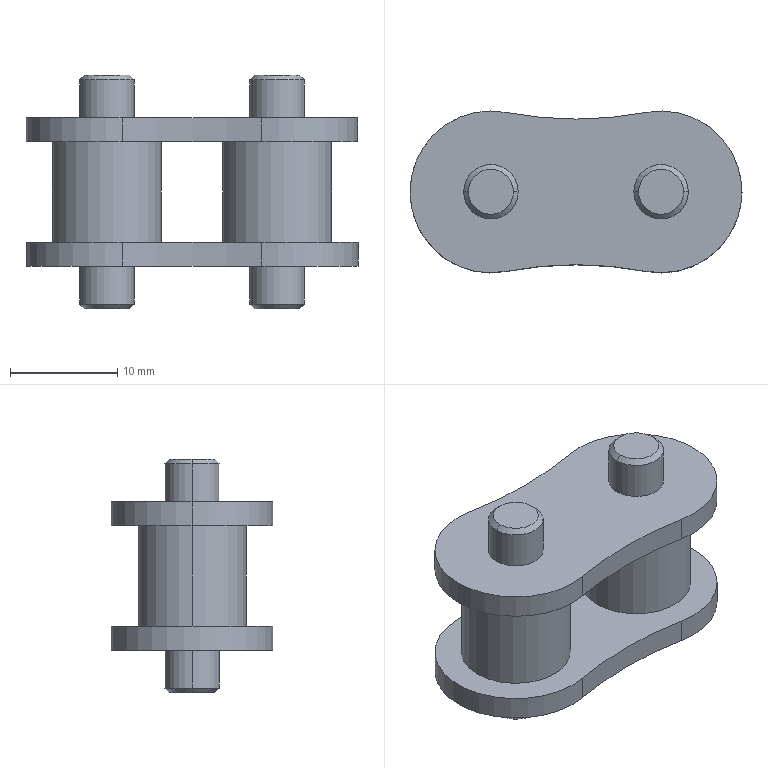Part | SolidWorks | features Boss 2, Chamfer 1, CompositeCurve 1, Extrusion 1, MirrorPattern 1 | 1 solid | 38 faces | box 30.965 x 15.09 x 21.8 mm | volume 3635 mm3 | cylinder 22 | cone 8 | plane 8 | commonest cylinder face diameters 5.09 x8 15.09 x6 10.16 x4 69.169 x4
STEP:
#1=CARTESIAN_POINT('',(-5.836,0.,10.9));
#2=VERTEX_POINT('',#1);
#3=CARTESIAN_POINT('',(-10.039,0.,10.9));
#4=VERTEX_POINT('',#3);
#5=CARTESIAN_POINT('',(-7.938,0.,10.9));
#6=DIRECTION('',(0.,0.,1.));
#7=DIRECTION('',(1.,0.,0.));
#8=AXIS2_PLACEMENT_3D('',#5,#6,#7);
#9=CIRCLE('',#8,2.101);
#10=EDGE_CURVE('',#2,#4,#9,.T.);
#11=ORIENTED_EDGE('',*,*,#10,.F.);
#12=CARTESIAN_POINT('',(-5.393,0.,10.456));
#13=VERTEX_POINT('',#12);
#14=CARTESIAN_POINT('',(-5.836,0.,10.9));
#15=DIRECTION('',(0.7071,0.,-0.7071));
#16=VECTOR('',#15,1000.);
#17=LINE('',#14,#16);
#18=EDGE_CURVE('',#2,#13,#17,.T.);
#19=ORIENTED_EDGE('',*,*,#18,.T.);
#20=CARTESIAN_POINT('',(-10.482,0.,10.456));
#21=VERTEX_POINT('',#20);
#22=CARTESIAN_POINT('',(-7.938,0.,10.456));
#23=DIRECTION('',(0.,0.,-1.));
#24=DIRECTION('',(1.,0.,0.));
#25=AXIS2_PLACEMENT_3D('',#22,#23,#24);
#26=CIRCLE('',#25,2.545);
#27=EDGE_CURVE('',#21,#13,#26,.T.);
#28=ORIENTED_EDGE('',*,*,#27,.F.);
#29=CARTESIAN_POINT('',(-10.039,0.,10.9));
#30=DIRECTION('',(-0.7071,0.,-0.7071));
#31=VECTOR('',#30,1000.);
#32=LINE('',#29,#31);
#33=EDGE_CURVE('',#4,#21,#32,.T.);
#34=ORIENTED_EDGE('',*,*,#33,.F.);
#35=EDGE_LOOP('',(#11,#19,#28,#34));
#36=FACE_OUTER_BOUND('',#35,.T.);
#37=CARTESIAN_POINT('',(-7.938,0.,10.9));
#38=DIRECTION('',(0.,0.,-1.));
#39=DIRECTION('',(-1.,0.,0.));
#40=AXIS2_PLACEMENT_3D('',#37,#38,#39);
#41=CONICAL_SURFACE('',#40,2.101,0.7854);
#42=ADVANCED_FACE('',(#36),#41,.T.);
#43=CARTESIAN_POINT('',(-10.038,0.,-10.9));
#44=VERTEX_POINT('',#43);
#45=CARTESIAN_POINT('',(-5.837,0.,-10.9));
#46=VERTEX_POINT('',#45);
#47=CARTESIAN_POINT('',(-7.938,0.,-10.9));
#48=DIRECTION('',(0.,0.,-1.));
#49=DIRECTION('',(1.,0.,0.));
#50=AXIS2_PLACEMENT_3D('',#47,#48,#49);
#51=CIRCLE('',#50,2.101);
#52=EDGE_CURVE('',#44,#46,#51,.T.);
#53=ORIENTED_EDGE('',*,*,#52,.F.);
#54=CARTESIAN_POINT('',(-10.482,0.,-10.456));
#55=VERTEX_POINT('',#54);
#56=CARTESIAN_POINT('',(-10.482,0.,-10.456));
#57=DIRECTION('',(-0.7071,0.,0.7071));
#58=VECTOR('',#57,1000.);
#59=LINE('',#56,#58);
#60=EDGE_CURVE('',#44,#55,#59,.T.);
#61=ORIENTED_EDGE('',*,*,#60,.T.);
#62=CARTESIAN_POINT('',(-5.393,0.,-10.456));
#63=VERTEX_POINT('',#62);
#64=CARTESIAN_POINT('',(-7.938,0.,-10.456));
#65=DIRECTION('',(0.,0.,1.));
#66=DIRECTION('',(1.,0.,0.));
#67=AXIS2_PLACEMENT_3D('',#64,#65,#66);
#68=CIRCLE('',#67,2.545);
#69=EDGE_CURVE('',#63,#55,#68,.T.);
#70=ORIENTED_EDGE('',*,*,#69,.F.);
#71=CARTESIAN_POINT('',(-5.393,0.,-10.456));
#72=DIRECTION('',(0.7071,0.,0.7071));
#73=VECTOR('',#72,1000.);
#74=LINE('',#71,#73);
#75=EDGE_CURVE('',#46,#63,#74,.T.);
#76=ORIENTED_EDGE('',*,*,#75,.F.);
#77=EDGE_LOOP('',(#53,#61,#70,#76));
#78=FACE_OUTER_BOUND('',#77,.T.);
#79=CARTESIAN_POINT('',(-7.938,0.,-10.456));
#80=DIRECTION('',(0.,0.,1.));
#81=DIRECTION('',(1.,0.,0.));
#82=AXIS2_PLACEMENT_3D('',#79,#80,#81);
#83=CONICAL_SURFACE('',#82,2.545,0.7854);
#84=ADVANCED_FACE('',(#78),#83,.T.);
#85=CARTESIAN_POINT('',(10.039,0.,10.9));
#86=VERTEX_POINT('',#85);
#87=CARTESIAN_POINT('',(5.836,0.,10.9));
#88=VERTEX_POINT('',#87);
#89=CARTESIAN_POINT('',(7.938,0.,10.9));
#90=DIRECTION('',(0.,0.,1.));
#91=DIRECTION('',(1.,0.,0.));
#92=AXIS2_PLACEMENT_3D('',#89,#90,#91);
#93=CIRCLE('',#92,2.101);
#94=EDGE_CURVE('',#86,#88,#93,.T.);
#95=ORIENTED_EDGE('',*,*,#94,.F.);
#96=CARTESIAN_POINT('',(10.482,0.,10.456));
#97=VERTEX_POINT('',#96);
#98=CARTESIAN_POINT('',(10.039,0.,10.9));
#99=DIRECTION('',(0.7071,0.,-0.7071));
#100=VECTOR('',#99,1000.);
#101=LINE('',#98,#100);
#102=EDGE_CURVE('',#86,#97,#101,.T.);
#103=ORIENTED_EDGE('',*,*,#102,.T.);
#104=CARTESIAN_POINT('',(5.393,0.,10.456));
#105=VERTEX_POINT('',#104);
#106=CARTESIAN_POINT('',(7.938,0.,10.456));
#107=DIRECTION('',(0.,0.,-1.));
#108=DIRECTION('',(1.,0.,0.));
#109=AXIS2_PLACEMENT_3D('',#106,#107,#108);
#110=CIRCLE('',#109,2.545);
#111=EDGE_CURVE('',#105,#97,#110,.T.);
#112=ORIENTED_EDGE('',*,*,#111,.F.);
#113=CARTESIAN_POINT('',(5.836,0.,10.9));
#114=DIRECTION('',(-0.7071,0.,-0.7071));
#115=VECTOR('',#114,1000.);
#116=LINE('',#113,#115);
#117=EDGE_CURVE('',#88,#105,#116,.T.);
#118=ORIENTED_EDGE('',*,*,#117,.F.);
#119=EDGE_LOOP('',(#95,#103,#112,#118));
#120=FACE_OUTER_BOUND('',#119,.T.);
#121=CARTESIAN_POINT('',(7.938,0.,10.9));
#122=DIRECTION('',(0.,0.,-1.));
#123=DIRECTION('',(-1.,0.,0.));
#124=AXIS2_PLACEMENT_3D('',#121,#122,#123);
#125=CONICAL_SURFACE('',#124,2.101,0.7854);
#126=ADVANCED_FACE('',(#120),#125,.T.);
#127=CARTESIAN_POINT('',(5.837,0.,-10.9));
#128=VERTEX_POINT('',#127);
#129=CARTESIAN_POINT('',(10.038,0.,-10.9));
#130=VERTEX_POINT('',#129);
#131=CARTESIAN_POINT('',(7.938,0.,-10.9));
#132=DIRECTION('',(0.,0.,-1.));
#133=DIRECTION('',(1.,0.,0.));
#134=AXIS2_PLACEMENT_3D('',#131,#132,#133);
#135=CIRCLE('',#134,2.101);
#136=EDGE_CURVE('',#128,#130,#135,.T.);
#137=ORIENTED_EDGE('',*,*,#136,.F.);
#138=CARTESIAN_POINT('',(5.393,0.,-10.456));
#139=VERTEX_POINT('',#138);
#140=CARTESIAN_POINT('',(5.393,0.,-10.456));
#141=DIRECTION('',(-0.7071,0.,0.7071));
#142=VECTOR('',#141,1000.);
#143=LINE('',#140,#142);
#144=EDGE_CURVE('',#128,#139,#143,.T.);
#145=ORIENTED_EDGE('',*,*,#144,.T.);
#146=CARTESIAN_POINT('',(10.482,0.,-10.456));
#147=VERTEX_POINT('',#146);
#148=CARTESIAN_POINT('',(7.938,0.,-10.456));
#149=DIRECTION('',(0.,0.,1.));
#150=DIRECTION('',(1.,0.,0.));
#151=AXIS2_PLACEMENT_3D('',#148,#149,#150);
#152=CIRCLE('',#151,2.545);
#153=EDGE_CURVE('',#147,#139,#152,.T.);
#154=ORIENTED_EDGE('',*,*,#153,.F.);
#155=CARTESIAN_POINT('',(10.482,0.,-10.456));
#156=DIRECTION('',(0.7071,0.,0.7071));
#157=VECTOR('',#156,1000.);
#158=LINE('',#155,#157);
#159=EDGE_CURVE('',#130,#147,#158,.T.);
#160=ORIENTED_EDGE('',*,*,#159,.F.);
#161=EDGE_LOOP('',(#137,#145,#154,#160));
#162=FACE_OUTER_BOUND('',#161,.T.);
#163=CARTESIAN_POINT('',(7.938,0.,-10.456));
#164=DIRECTION('',(0.,0.,1.));
#165=DIRECTION('',(1.,0.,0.));
#166=AXIS2_PLACEMENT_3D('',#163,#164,#165);
#167=CONICAL_SURFACE('',#166,2.545,0.7854);
#168=ADVANCED_FACE('',(#162),#167,.T.);
#169=CARTESIAN_POINT('',(-5.393,0.,6.92));
#170=VERTEX_POINT('',#169);
#171=CARTESIAN_POINT('',(-10.482,0.,6.92));
#172=VERTEX_POINT('',#171);
#173=CARTESIAN_POINT('',(-7.938,0.,6.92));
#174=DIRECTION('',(0.,0.,1.));
#175=DIRECTION('',(1.,0.,0.));
#176=AXIS2_PLACEMENT_3D('',#173,#174,#175);
#177=CIRCLE('',#176,2.545);
#178=EDGE_CURVE('',#170,#172,#177,.T.);
#179=ORIENTED_EDGE('',*,*,#178,.T.);
#180=CARTESIAN_POINT('',(-10.482,0.,-10.9));
#181=DIRECTION('',(0.,0.,1.));
#182=VECTOR('',#181,1000.);
#183=LINE('',#180,#182);
#184=EDGE_CURVE('',#172,#21,#183,.T.);
#185=ORIENTED_EDGE('',*,*,#184,.T.);
#186=ORIENTED_EDGE('',*,*,#27,.T.);
#187=CARTESIAN_POINT('',(-5.393,0.,-10.9));
#188=DIRECTION('',(0.,0.,1.));
#189=VECTOR('',#188,1000.);
#190=LINE('',#187,#189);
#191=EDGE_CURVE('',#170,#13,#190,.T.);
#192=ORIENTED_EDGE('',*,*,#191,.F.);
#193=EDGE_LOOP('',(#179,#185,#186,#192));
#194=FACE_OUTER_BOUND('',#193,.T.);
#195=CARTESIAN_POINT('',(-7.938,0.,-10.9));
#196=DIRECTION('',(0.,0.,1.));
#197=DIRECTION('',(1.,0.,0.));
#198=AXIS2_PLACEMENT_3D('',#195,#196,#197);
#199=CYLINDRICAL_SURFACE('',#198,2.545);
#200=ADVANCED_FACE('',(#194),#199,.T.);
#201=ORIENTED_EDGE('',*,*,#69,.T.);
#202=CARTESIAN_POINT('',(-10.482,0.,-6.92));
#203=VERTEX_POINT('',#202);
#204=CARTESIAN_POINT('',(-10.482,0.,-10.9));
#205=DIRECTION('',(0.,0.,1.));
#206=VECTOR('',#205,1000.);
#207=LINE('',#204,#206);
#208=EDGE_CURVE('',#55,#203,#207,.T.);
#209=ORIENTED_EDGE('',*,*,#208,.T.);
#210=CARTESIAN_POINT('',(-5.393,0.,-6.92));
#211=VERTEX_POINT('',#210);
#212=CARTESIAN_POINT('',(-7.938,0.,-6.92));
#213=DIRECTION('',(0.,0.,-1.));
#214=DIRECTION('',(-1.,0.,0.));
#215=AXIS2_PLACEMENT_3D('',#212,#213,#214);
#216=CIRCLE('',#215,2.545);
#217=EDGE_CURVE('',#203,#211,#216,.T.);
#218=ORIENTED_EDGE('',*,*,#217,.T.);
#219=CARTESIAN_POINT('',(-5.393,0.,-10.9));
#220=DIRECTION('',(0.,0.,1.));
#221=VECTOR('',#220,1000.);
#222=LINE('',#219,#221);
#223=EDGE_CURVE('',#63,#211,#222,.T.);
#224=ORIENTED_EDGE('',*,*,#223,.F.);
#225=EDGE_LOOP('',(#201,#209,#218,#224));
#226=FACE_OUTER_BOUND('',#225,.T.);
#227=CARTESIAN_POINT('',(-7.938,0.,-10.9));
#228=DIRECTION('',(0.,0.,1.));
#229=DIRECTION('',(1.,0.,0.));
#230=AXIS2_PLACEMENT_3D('',#227,#228,#229);
#231=CYLINDRICAL_SURFACE('',#230,2.545);
#232=ADVANCED_FACE('',(#226),#231,.T.);
#233=CARTESIAN_POINT('',(10.482,0.,6.92));
#234=VERTEX_POINT('',#233);
#235=CARTESIAN_POINT('',(5.393,0.,6.92));
#236=VERTEX_POINT('',#235);
#237=CARTESIAN_POINT('',(7.938,0.,6.92));
#238=DIRECTION('',(0.,0.,1.));
#239=DIRECTION('',(1.,0.,0.));
#240=AXIS2_PLACEMENT_3D('',#237,#238,#239);
#241=CIRCLE('',#240,2.545);
#242=EDGE_CURVE('',#234,#236,#241,.T.);
#243=ORIENTED_EDGE('',*,*,#242,.T.);
#244=CARTESIAN_POINT('',(5.393,0.,-10.9));
#245=DIRECTION('',(0.,0.,1.));
#246=VECTOR('',#245,1000.);
#247=LINE('',#244,#246);
#248=EDGE_CURVE('',#236,#105,#247,.T.);
#249=ORIENTED_EDGE('',*,*,#248,.T.);
#250=ORIENTED_EDGE('',*,*,#111,.T.);
#251=CARTESIAN_POINT('',(10.482,0.,-10.9));
#252=DIRECTION('',(0.,0.,1.));
#253=VECTOR('',#252,1000.);
#254=LINE('',#251,#253);
#255=EDGE_CURVE('',#234,#97,#254,.T.);
#256=ORIENTED_EDGE('',*,*,#255,.F.);
#257=EDGE_LOOP('',(#243,#249,#250,#256));
#258=FACE_OUTER_BOUND('',#257,.T.);
#259=CARTESIAN_POINT('',(7.938,0.,-10.9));
#260=DIRECTION('',(0.,0.,1.));
#261=DIRECTION('',(1.,0.,0.));
#262=AXIS2_PLACEMENT_3D('',#259,#260,#261);
#263=CYLINDRICAL_SURFACE('',#262,2.545);
#264=ADVANCED_FACE('',(#258),#263,.T.);
#265=ORIENTED_EDGE('',*,*,#153,.T.);
#266=CARTESIAN_POINT('',(5.393,0.,-6.92));
#267=VERTEX_POINT('',#266);
#268=CARTESIAN_POINT('',(5.393,0.,-10.9));
#269=DIRECTION('',(0.,0.,1.));
#270=VECTOR('',#269,1000.);
#271=LINE('',#268,#270);
#272=EDGE_CURVE('',#139,#267,#271,.T.);
#273=ORIENTED_EDGE('',*,*,#272,.T.);
#274=CARTESIAN_POINT('',(10.482,0.,-6.92));
#275=VERTEX_POINT('',#274);
#276=CARTESIAN_POINT('',(7.938,0.,-6.92));
#277=DIRECTION('',(0.,0.,-1.));
#278=DIRECTION('',(-1.,0.,0.));
#279=AXIS2_PLACEMENT_3D('',#276,#277,#278);
#280=CIRCLE('',#279,2.545);
#281=EDGE_CURVE('',#267,#275,#280,.T.);
#282=ORIENTED_EDGE('',*,*,#281,.T.);
#283=CARTESIAN_POINT('',(10.482,0.,-10.9));
#284=DIRECTION('',(0.,0.,1.));
#285=VECTOR('',#284,1000.);
#286=LINE('',#283,#285);
#287=EDGE_CURVE('',#147,#275,#286,.T.);
#288=ORIENTED_EDGE('',*,*,#287,.F.);
#289=EDGE_LOOP('',(#265,#273,#282,#288));
#290=FACE_OUTER_BOUND('',#289,.T.);
#291=CARTESIAN_POINT('',(7.938,0.,-10.9));
#292=DIRECTION('',(0.,0.,1.));
#293=DIRECTION('',(1.,0.,0.));
#294=AXIS2_PLACEMENT_3D('',#291,#292,#293);
#295=CYLINDRICAL_SURFACE('',#294,2.545);
#296=ADVANCED_FACE('',(#290),#295,.T.);
#297=CARTESIAN_POINT('',(6.516,-7.41,-6.92));
#298=VERTEX_POINT('',#297);
#299=CARTESIAN_POINT('',(15.482,0.,-6.92));
#300=VERTEX_POINT('',#299);
#301=CARTESIAN_POINT('',(7.938,0.,-6.92));
#302=DIRECTION('',(0.,0.,1.));
#303=DIRECTION('',(1.,0.,0.));
#304=AXIS2_PLACEMENT_3D('',#301,#302,#303);
#305=CIRCLE('',#304,7.545);
#306=EDGE_CURVE('',#298,#300,#305,.T.);
#307=ORIENTED_EDGE('',*,*,#306,.T.);
#308=CARTESIAN_POINT('',(15.482,0.,-4.7));
#309=VERTEX_POINT('',#308);
#310=CARTESIAN_POINT('',(15.482,0.,-6.92));
#311=DIRECTION('',(0.,0.,1.));
#312=VECTOR('',#311,1000.);
#313=LINE('',#310,#312);
#314=EDGE_CURVE('',#300,#309,#313,.T.);
#315=ORIENTED_EDGE('',*,*,#314,.T.);
#316=CARTESIAN_POINT('',(6.516,-7.41,-4.7));
#317=VERTEX_POINT('',#316);
#318=CARTESIAN_POINT('',(7.938,0.,-4.7));
#319=DIRECTION('',(0.,0.,1.));
#320=DIRECTION('',(1.,0.,0.));
#321=AXIS2_PLACEMENT_3D('',#318,#319,#320);
#322=CIRCLE('',#321,7.545);
#323=EDGE_CURVE('',#317,#309,#322,.T.);
#324=ORIENTED_EDGE('',*,*,#323,.F.);
#325=CARTESIAN_POINT('',(6.516,-7.41,-6.92));
#326=DIRECTION('',(0.,0.,1.));
#327=VECTOR('',#326,1000.);
#328=LINE('',#325,#327);
#329=EDGE_CURVE('',#298,#317,#328,.T.);
#330=ORIENTED_EDGE('',*,*,#329,.F.);
#331=EDGE_LOOP('',(#307,#315,#324,#330));
#332=FACE_OUTER_BOUND('',#331,.T.);
#333=CARTESIAN_POINT('',(7.938,0.,-6.92));
#334=DIRECTION('',(0.,0.,1.));
#335=DIRECTION('',(1.,0.,0.));
#336=AXIS2_PLACEMENT_3D('',#333,#334,#335);
#337=CYLINDRICAL_SURFACE('',#336,7.545);
#338=ADVANCED_FACE('',(#332),#337,.T.);
#339=CARTESIAN_POINT('',(-13.018,0.,4.7));
#340=VERTEX_POINT('',#339);
#341=CARTESIAN_POINT('',(-2.857,0.,4.7));
#342=VERTEX_POINT('',#341);
#343=CARTESIAN_POINT('',(-7.938,0.,4.7));
#344=DIRECTION('',(0.,0.,-1.));
#345=DIRECTION('',(1.,0.,0.));
#346=AXIS2_PLACEMENT_3D('',#343,#344,#345);
#347=CIRCLE('',#346,5.08);
#348=EDGE_CURVE('',#340,#342,#347,.T.);
#349=ORIENTED_EDGE('',*,*,#348,.T.);
#350=CARTESIAN_POINT('',(-2.857,0.,-4.7));
#351=VERTEX_POINT('',#350);
#352=CARTESIAN_POINT('',(-2.857,0.,4.7));
#353=DIRECTION('',(0.,0.,-1.));
#354=VECTOR('',#353,1000.);
#355=LINE('',#352,#354);
#356=EDGE_CURVE('',#342,#351,#355,.T.);
#357=ORIENTED_EDGE('',*,*,#356,.T.);
#358=CARTESIAN_POINT('',(-13.018,0.,-4.7));
#359=VERTEX_POINT('',#358);
#360=CARTESIAN_POINT('',(-7.938,0.,-4.7));
#361=DIRECTION('',(0.,0.,-1.));
#362=DIRECTION('',(-1.,0.,0.));
#363=AXIS2_PLACEMENT_3D('',#360,#361,#362);
#364=CIRCLE('',#363,5.08);
#365=EDGE_CURVE('',#359,#351,#364,.T.);
#366=ORIENTED_EDGE('',*,*,#365,.F.);
#367=CARTESIAN_POINT('',(-13.018,0.,4.7));
#368=DIRECTION('',(0.,0.,-1.));
#369=VECTOR('',#368,1000.);
#370=LINE('',#367,#369);
#371=EDGE_CURVE('',#340,#359,#370,.T.);
#372=ORIENTED_EDGE('',*,*,#371,.F.);
#373=EDGE_LOOP('',(#349,#357,#366,#372));
#374=FACE_OUTER_BOUND('',#373,.T.);
#375=CARTESIAN_POINT('',(-7.938,0.,4.7));
#376=DIRECTION('',(0.,0.,-1.));
#377=DIRECTION('',(-1.,0.,0.));
#378=AXIS2_PLACEMENT_3D('',#375,#376,#377);
#379=CYLINDRICAL_SURFACE('',#378,5.08);
#380=ADVANCED_FACE('',(#374),#379,.T.);
#381=CARTESIAN_POINT('',(-15.482,0.,6.92));
#382=VERTEX_POINT('',#381);
#383=CARTESIAN_POINT('',(-6.516,-7.41,6.92));
#384=VERTEX_POINT('',#383);
#385=CARTESIAN_POINT('',(-7.938,0.,6.92));
#386=DIRECTION('',(0.,0.,1.));
#387=DIRECTION('',(1.,0.,0.));
#388=AXIS2_PLACEMENT_3D('',#385,#386,#387);
#389=CIRCLE('',#388,7.545);
#390=EDGE_CURVE('',#382,#384,#389,.T.);
#391=ORIENTED_EDGE('',*,*,#390,.F.);
#392=CARTESIAN_POINT('',(-15.482,0.,4.7));
#393=VERTEX_POINT('',#392);
#394=CARTESIAN_POINT('',(-15.482,0.,6.92));
#395=DIRECTION('',(0.,0.,-1.));
#396=VECTOR('',#395,1000.);
#397=LINE('',#394,#396);
#398=EDGE_CURVE('',#382,#393,#397,.T.);
#399=ORIENTED_EDGE('',*,*,#398,.T.);
#400=CARTESIAN_POINT('',(-6.516,-7.41,4.7));
#401=VERTEX_POINT('',#400);
#402=CARTESIAN_POINT('',(-7.938,0.,4.7));
#403=DIRECTION('',(0.,0.,1.));
#404=DIRECTION('',(1.,0.,0.));
#405=AXIS2_PLACEMENT_3D('',#402,#403,#404);
#406=CIRCLE('',#405,7.545);
#407=EDGE_CURVE('',#393,#401,#406,.T.);
#408=ORIENTED_EDGE('',*,*,#407,.T.);
#409=CARTESIAN_POINT('',(-6.516,-7.41,6.92));
#410=DIRECTION('',(0.,0.,-1.));
#411=VECTOR('',#410,1000.);
#412=LINE('',#409,#411);
#413=EDGE_CURVE('',#384,#401,#412,.T.);
#414=ORIENTED_EDGE('',*,*,#413,.F.);
#415=EDGE_LOOP('',(#391,#399,#408,#414));
#416=FACE_OUTER_BOUND('',#415,.T.);
#417=CARTESIAN_POINT('',(-7.938,0.,6.92));
#418=DIRECTION('',(0.,0.,-1.));
#419=DIRECTION('',(-1.,0.,0.));
#420=AXIS2_PLACEMENT_3D('',#417,#418,#419);
#421=CYLINDRICAL_SURFACE('',#420,7.545);
#422=ADVANCED_FACE('',(#416),#421,.T.);
#423=CARTESIAN_POINT('',(13.018,0.,4.7));
#424=VERTEX_POINT('',#423);
#425=CARTESIAN_POINT('',(2.857,0.,4.7));
#426=VERTEX_POINT('',#425);
#427=CARTESIAN_POINT('',(7.938,0.,4.7));
#428=DIRECTION('',(0.,0.,1.));
#429=DIRECTION('',(1.,0.,0.));
#430=AXIS2_PLACEMENT_3D('',#427,#428,#429);
#431=CIRCLE('',#430,5.08);
#432=EDGE_CURVE('',#424,#426,#431,.T.);
#433=ORIENTED_EDGE('',*,*,#432,.F.);
#434=CARTESIAN_POINT('',(13.018,0.,-4.7));
#435=VERTEX_POINT('',#434);
#436=CARTESIAN_POINT('',(13.018,0.,4.7));
#437=DIRECTION('',(0.,0.,-1.));
#438=VECTOR('',#437,1000.);
#439=LINE('',#436,#438);
#440=EDGE_CURVE('',#424,#435,#439,.T.);
#441=ORIENTED_EDGE('',*,*,#440,.T.);
#442=CARTESIAN_POINT('',(2.857,0.,-4.7));
#443=VERTEX_POINT('',#442);
#444=CARTESIAN_POINT('',(7.938,0.,-4.7));
#445=DIRECTION('',(0.,0.,-1.));
#446=DIRECTION('',(-1.,0.,0.));
#447=AXIS2_PLACEMENT_3D('',#444,#445,#446);
#448=CIRCLE('',#447,5.08);
#449=EDGE_CURVE('',#443,#435,#448,.T.);
#450=ORIENTED_EDGE('',*,*,#449,.F.);
#451=CARTESIAN_POINT('',(2.857,0.,4.7));
#452=DIRECTION('',(0.,0.,-1.));
#453=VECTOR('',#452,1000.);
#454=LINE('',#451,#453);
#455=EDGE_CURVE('',#426,#443,#454,.T.);
#456=ORIENTED_EDGE('',*,*,#455,.F.);
#457=EDGE_LOOP('',(#433,#441,#450,#456));
#458=FACE_OUTER_BOUND('',#457,.T.);
#459=CARTESIAN_POINT('',(7.938,0.,4.7));
#460=DIRECTION('',(0.,0.,-1.));
#461=DIRECTION('',(-1.,0.,0.));
#462=AXIS2_PLACEMENT_3D('',#459,#460,#461);
#463=CYLINDRICAL_SURFACE('',#462,5.08);
#464=ADVANCED_FACE('',(#458),#463,.T.);
#465=CARTESIAN_POINT('',(6.516,-7.41,4.7));
#466=VERTEX_POINT('',#465);
#467=CARTESIAN_POINT('',(0.,-41.375,4.7));
#468=DIRECTION('',(0.,0.,-1.));
#469=DIRECTION('',(1.,0.,0.));
#470=AXIS2_PLACEMENT_3D('',#467,#468,#469);
#471=CIRCLE('',#470,34.584);
#472=EDGE_CURVE('',#401,#466,#471,.T.);
#473=ORIENTED_EDGE('',*,*,#472,.F.);
#474=ORIENTED_EDGE('',*,*,#407,.F.);
#475=CARTESIAN_POINT('',(-6.516,7.41,4.7));
#476=VERTEX_POINT('',#475);
#477=CARTESIAN_POINT('',(-7.938,0.,4.7));
#478=DIRECTION('',(0.,0.,1.));
#479=DIRECTION('',(1.,0.,0.));
#480=AXIS2_PLACEMENT_3D('',#477,#478,#479);
#481=CIRCLE('',#480,7.545);
#482=EDGE_CURVE('',#476,#393,#481,.T.);
#483=ORIENTED_EDGE('',*,*,#482,.F.);
#484=CARTESIAN_POINT('',(6.516,7.41,4.7));
#485=VERTEX_POINT('',#484);
#486=CARTESIAN_POINT('',(0.,41.375,4.7));
#487=DIRECTION('',(0.,0.,-1.));
#488=DIRECTION('',(1.,0.,0.));
#489=AXIS2_PLACEMENT_3D('',#486,#487,#488);
#490=CIRCLE('',#489,34.584);
#491=EDGE_CURVE('',#485,#476,#490,.T.);
#492=ORIENTED_EDGE('',*,*,#491,.F.);
#493=CARTESIAN_POINT('',(7.938,0.,4.7));
#494=DIRECTION('',(0.,0.,1.));
#495=DIRECTION('',(1.,0.,0.));
#496=AXIS2_PLACEMENT_3D('',#493,#494,#495);
#497=CIRCLE('',#496,7.545);
#498=EDGE_CURVE('',#466,#485,#497,.T.);
#499=ORIENTED_EDGE('',*,*,#498,.F.);
#500=EDGE_LOOP('',(#473,#474,#483,#492,#499));
#501=FACE_OUTER_BOUND('',#500,.T.);
#502=CARTESIAN_POINT('',(7.938,0.,4.7));
#503=DIRECTION('',(0.,0.,1.));
#504=DIRECTION('',(1.,0.,0.));
#505=AXIS2_PLACEMENT_3D('',#502,#503,#504);
#506=CIRCLE('',#505,5.08);
#507=EDGE_CURVE('',#426,#424,#506,.T.);
#508=ORIENTED_EDGE('',*,*,#507,.T.);
#509=ORIENTED_EDGE('',*,*,#432,.T.);
#510=EDGE_LOOP('',(#508,#509));
#511=FACE_BOUND('',#510,.T.);
#512=ORIENTED_EDGE('',*,*,#348,.F.);
#513=CARTESIAN_POINT('',(-7.938,0.,4.7));
#514=DIRECTION('',(0.,0.,-1.));
#515=DIRECTION('',(1.,0.,0.));
#516=AXIS2_PLACEMENT_3D('',#513,#514,#515);
#517=CIRCLE('',#516,5.08);
#518=EDGE_CURVE('',#342,#340,#517,.T.);
#519=ORIENTED_EDGE('',*,*,#518,.F.);
#520=EDGE_LOOP('',(#512,#519));
#521=FACE_BOUND('',#520,.T.);
#522=CARTESIAN_POINT('',(-3.969,-20.687,4.7));
#523=DIRECTION('',(0.,0.,1.));
#524=DIRECTION('',(1.,0.,0.));
#525=AXIS2_PLACEMENT_3D('',#522,#523,#524);
#526=PLANE('',#525);
#527=ADVANCED_FACE('',(#501,#511,#521),#526,.F.);
#528=ORIENTED_EDGE('',*,*,#440,.F.);
#529=ORIENTED_EDGE('',*,*,#507,.F.);
#530=ORIENTED_EDGE('',*,*,#455,.T.);
#531=CARTESIAN_POINT('',(7.938,0.,-4.7));
#532=DIRECTION('',(0.,0.,-1.));
#533=DIRECTION('',(-1.,0.,0.));
#534=AXIS2_PLACEMENT_3D('',#531,#532,#533);
#535=CIRCLE('',#534,5.08);
#536=EDGE_CURVE('',#435,#443,#535,.T.);
#537=ORIENTED_EDGE('',*,*,#536,.F.);
#538=EDGE_LOOP('',(#528,#529,#530,#537));
#539=FACE_OUTER_BOUND('',#538,.T.);
#540=CARTESIAN_POINT('',(7.938,0.,4.7));
#541=DIRECTION('',(0.,0.,-1.));
#542=DIRECTION('',(-1.,0.,0.));
#543=AXIS2_PLACEMENT_3D('',#540,#541,#542);
#544=CYLINDRICAL_SURFACE('',#543,5.08);
#545=ADVANCED_FACE('',(#539),#544,.T.);
#546=ORIENTED_EDGE('',*,*,#472,.T.);
#547=CARTESIAN_POINT('',(6.516,-7.41,6.92));
#548=VERTEX_POINT('',#547);
#549=CARTESIAN_POINT('',(6.516,-7.41,6.92));
#550=DIRECTION('',(0.,0.,-1.));
#551=VECTOR('',#550,1000.);
#552=LINE('',#549,#551);
#553=EDGE_CURVE('',#548,#466,#552,.T.);
#554=ORIENTED_EDGE('',*,*,#553,.F.);
#555=CARTESIAN_POINT('',(0.,-41.375,6.92));
#556=DIRECTION('',(0.,0.,-1.));
#557=DIRECTION('',(1.,0.,0.));
#558=AXIS2_PLACEMENT_3D('',#555,#556,#557);
#559=CIRCLE('',#558,34.584);
#560=EDGE_CURVE('',#384,#548,#559,.T.);
#561=ORIENTED_EDGE('',*,*,#560,.F.);
#562=ORIENTED_EDGE('',*,*,#413,.T.);
#563=EDGE_LOOP('',(#546,#554,#561,#562));
#564=FACE_OUTER_BOUND('',#563,.T.);
#565=CARTESIAN_POINT('',(0.,-41.375,6.92));
#566=DIRECTION('',(0.,0.,-1.));
#567=DIRECTION('',(-1.,0.,0.));
#568=AXIS2_PLACEMENT_3D('',#565,#566,#567);
#569=CYLINDRICAL_SURFACE('',#568,34.584);
#570=ADVANCED_FACE('',(#564),#569,.F.);
#571=ORIENTED_EDGE('',*,*,#498,.T.);
#572=CARTESIAN_POINT('',(6.516,7.41,6.92));
#573=VERTEX_POINT('',#572);
#574=CARTESIAN_POINT('',(6.516,7.41,6.92));
#575=DIRECTION('',(0.,0.,-1.));
#576=VECTOR('',#575,1000.);
#577=LINE('',#574,#576);
#578=EDGE_CURVE('',#573,#485,#577,.T.);
#579=ORIENTED_EDGE('',*,*,#578,.F.);
#580=CARTESIAN_POINT('',(7.938,0.,6.92));
#581=DIRECTION('',(0.,0.,1.));
#582=DIRECTION('',(1.,0.,0.));
#583=AXIS2_PLACEMENT_3D('',#580,#581,#582);
#584=CIRCLE('',#583,7.545);
#585=EDGE_CURVE('',#548,#573,#584,.T.);
#586=ORIENTED_EDGE('',*,*,#585,.F.);
#587=ORIENTED_EDGE('',*,*,#553,.T.);
#588=EDGE_LOOP('',(#571,#579,#586,#587));
#589=FACE_OUTER_BOUND('',#588,.T.);
#590=CARTESIAN_POINT('',(7.938,0.,6.92));
#591=DIRECTION('',(0.,0.,-1.));
#592=DIRECTION('',(-1.,0.,0.));
#593=AXIS2_PLACEMENT_3D('',#590,#591,#592);
#594=CYLINDRICAL_SURFACE('',#593,7.545);
#595=ADVANCED_FACE('',(#589),#594,.T.);
#596=ORIENTED_EDGE('',*,*,#491,.T.);
#597=CARTESIAN_POINT('',(-6.516,7.41,6.92));
#598=VERTEX_POINT('',#597);
#599=CARTESIAN_POINT('',(-6.516,7.41,6.92));
#600=DIRECTION('',(0.,0.,-1.));
#601=VECTOR('',#600,1000.);
#602=LINE('',#599,#601);
#603=EDGE_CURVE('',#598,#476,#602,.T.);
#604=ORIENTED_EDGE('',*,*,#603,.F.);
#605=CARTESIAN_POINT('',(0.,41.375,6.92));
#606=DIRECTION('',(0.,0.,-1.));
#607=DIRECTION('',(1.,0.,0.));
#608=AXIS2_PLACEMENT_3D('',#605,#606,#607);
#609=CIRCLE('',#608,34.584);
#610=EDGE_CURVE('',#573,#598,#609,.T.);
#611=ORIENTED_EDGE('',*,*,#610,.F.);
#612=ORIENTED_EDGE('',*,*,#578,.T.);
#613=EDGE_LOOP('',(#596,#604,#611,#612));
#614=FACE_OUTER_BOUND('',#613,.T.);
#615=CARTESIAN_POINT('',(0.,41.375,6.92));
#616=DIRECTION('',(0.,0.,-1.));
#617=DIRECTION('',(-1.,0.,0.));
#618=AXIS2_PLACEMENT_3D('',#615,#616,#617);
#619=CYLINDRICAL_SURFACE('',#618,34.584);
#620=ADVANCED_FACE('',(#614),#619,.F.);
#621=ORIENTED_EDGE('',*,*,#398,.F.);
#622=CARTESIAN_POINT('',(-7.938,0.,6.92));
#623=DIRECTION('',(0.,0.,1.));
#624=DIRECTION('',(1.,0.,0.));
#625=AXIS2_PLACEMENT_3D('',#622,#623,#624);
#626=CIRCLE('',#625,7.545);
#627=EDGE_CURVE('',#598,#382,#626,.T.);
#628=ORIENTED_EDGE('',*,*,#627,.F.);
#629=ORIENTED_EDGE('',*,*,#603,.T.);
#630=ORIENTED_EDGE('',*,*,#482,.T.);
#631=EDGE_LOOP('',(#621,#628,#629,#630));
#632=FACE_OUTER_BOUND('',#631,.T.);
#633=CARTESIAN_POINT('',(-7.938,0.,6.92));
#634=DIRECTION('',(0.,0.,-1.));
#635=DIRECTION('',(-1.,0.,0.));
#636=AXIS2_PLACEMENT_3D('',#633,#634,#635);
#637=CYLINDRICAL_SURFACE('',#636,7.545);
#638=ADVANCED_FACE('',(#632),#637,.T.);
#639=ORIENTED_EDGE('',*,*,#178,.F.);
#640=CARTESIAN_POINT('',(-7.938,0.,6.92));
#641=DIRECTION('',(0.,0.,1.));
#642=DIRECTION('',(1.,0.,0.));
#643=AXIS2_PLACEMENT_3D('',#640,#641,#642);
#644=CIRCLE('',#643,2.545);
#645=EDGE_CURVE('',#172,#170,#644,.T.);
#646=ORIENTED_EDGE('',*,*,#645,.F.);
#647=EDGE_LOOP('',(#639,#646));
#648=FACE_BOUND('',#647,.T.);
#649=ORIENTED_EDGE('',*,*,#242,.F.);
#650=CARTESIAN_POINT('',(7.938,0.,6.92));
#651=DIRECTION('',(0.,0.,1.));
#652=DIRECTION('',(1.,0.,0.));
#653=AXIS2_PLACEMENT_3D('',#650,#651,#652);
#654=CIRCLE('',#653,2.545);
#655=EDGE_CURVE('',#236,#234,#654,.T.);
#656=ORIENTED_EDGE('',*,*,#655,.F.);
#657=EDGE_LOOP('',(#649,#656));
#658=FACE_BOUND('',#657,.T.);
#659=ORIENTED_EDGE('',*,*,#560,.T.);
#660=ORIENTED_EDGE('',*,*,#585,.T.);
#661=ORIENTED_EDGE('',*,*,#610,.T.);
#662=ORIENTED_EDGE('',*,*,#627,.T.);
#663=ORIENTED_EDGE('',*,*,#390,.T.);
#664=EDGE_LOOP('',(#659,#660,#661,#662,#663));
#665=FACE_OUTER_BOUND('',#664,.T.);
#666=CARTESIAN_POINT('',(-3.969,-20.687,6.92));
#667=DIRECTION('',(0.,0.,1.));
#668=DIRECTION('',(1.,0.,0.));
#669=AXIS2_PLACEMENT_3D('',#666,#667,#668);
#670=PLANE('',#669);
#671=ADVANCED_FACE('',(#648,#658,#665),#670,.T.);
#672=ORIENTED_EDGE('',*,*,#356,.F.);
#673=ORIENTED_EDGE('',*,*,#518,.T.);
#674=ORIENTED_EDGE('',*,*,#371,.T.);
#675=CARTESIAN_POINT('',(-7.938,0.,-4.7));
#676=DIRECTION('',(0.,0.,-1.));
#677=DIRECTION('',(-1.,0.,0.));
#678=AXIS2_PLACEMENT_3D('',#675,#676,#677);
#679=CIRCLE('',#678,5.08);
#680=EDGE_CURVE('',#351,#359,#679,.T.);
#681=ORIENTED_EDGE('',*,*,#680,.F.);
#682=EDGE_LOOP('',(#672,#673,#674,#681));
#683=FACE_OUTER_BOUND('',#682,.T.);
#684=CARTESIAN_POINT('',(-7.938,0.,4.7));
#685=DIRECTION('',(0.,0.,-1.));
#686=DIRECTION('',(-1.,0.,0.));
#687=AXIS2_PLACEMENT_3D('',#684,#685,#686);
#688=CYLINDRICAL_SURFACE('',#687,5.08);
#689=ADVANCED_FACE('',(#683),#688,.T.);
#690=ORIENTED_EDGE('',*,*,#365,.T.);
#691=ORIENTED_EDGE('',*,*,#680,.T.);
#692=EDGE_LOOP('',(#690,#691));
#693=FACE_BOUND('',#692,.T.);
#694=CARTESIAN_POINT('',(-6.516,-7.41,-4.7));
#695=VERTEX_POINT('',#694);
#696=CARTESIAN_POINT('',(0.,-41.375,-4.7));
#697=DIRECTION('',(0.,0.,-1.));
#698=DIRECTION('',(1.,0.,0.));
#699=AXIS2_PLACEMENT_3D('',#696,#697,#698);
#700=CIRCLE('',#699,34.584);
#701=EDGE_CURVE('',#695,#317,#700,.T.);
#702=ORIENTED_EDGE('',*,*,#701,.T.);
#703=ORIENTED_EDGE('',*,*,#323,.T.);
#704=CARTESIAN_POINT('',(6.516,7.41,-4.7));
#705=VERTEX_POINT('',#704);
#706=CARTESIAN_POINT('',(7.938,0.,-4.7));
#707=DIRECTION('',(0.,0.,1.));
#708=DIRECTION('',(1.,0.,0.));
#709=AXIS2_PLACEMENT_3D('',#706,#707,#708);
#710=CIRCLE('',#709,7.545);
#711=EDGE_CURVE('',#309,#705,#710,.T.);
#712=ORIENTED_EDGE('',*,*,#711,.T.);
#713=CARTESIAN_POINT('',(-6.516,7.41,-4.7));
#714=VERTEX_POINT('',#713);
#715=CARTESIAN_POINT('',(0.,41.375,-4.7));
#716=DIRECTION('',(0.,0.,-1.));
#717=DIRECTION('',(1.,0.,0.));
#718=AXIS2_PLACEMENT_3D('',#715,#716,#717);
#719=CIRCLE('',#718,34.584);
#720=EDGE_CURVE('',#705,#714,#719,.T.);
#721=ORIENTED_EDGE('',*,*,#720,.T.);
#722=CARTESIAN_POINT('',(-7.938,0.,-4.7));
#723=DIRECTION('',(0.,0.,1.));
#724=DIRECTION('',(1.,0.,0.));
#725=AXIS2_PLACEMENT_3D('',#722,#723,#724);
#726=CIRCLE('',#725,7.545);
#727=EDGE_CURVE('',#714,#695,#726,.T.);
#728=ORIENTED_EDGE('',*,*,#727,.T.);
#729=EDGE_LOOP('',(#702,#703,#712,#721,#728));
#730=FACE_OUTER_BOUND('',#729,.T.);
#731=ORIENTED_EDGE('',*,*,#449,.T.);
#732=ORIENTED_EDGE('',*,*,#536,.T.);
#733=EDGE_LOOP('',(#731,#732));
#734=FACE_BOUND('',#733,.T.);
#735=CARTESIAN_POINT('',(-3.969,-20.687,-4.7));
#736=DIRECTION('',(0.,0.,-1.));
#737=DIRECTION('',(1.,0.,0.));
#738=AXIS2_PLACEMENT_3D('',#735,#736,#737);
#739=PLANE('',#738);
#740=ADVANCED_FACE('',(#693,#730,#734),#739,.F.);
#741=ORIENTED_EDGE('',*,*,#701,.F.);
#742=CARTESIAN_POINT('',(-6.516,-7.41,-6.92));
#743=VERTEX_POINT('',#742);
#744=CARTESIAN_POINT('',(-6.516,-7.41,-6.92));
#745=DIRECTION('',(0.,0.,1.));
#746=VECTOR('',#745,1000.);
#747=LINE('',#744,#746);
#748=EDGE_CURVE('',#743,#695,#747,.T.);
#749=ORIENTED_EDGE('',*,*,#748,.F.);
#750=CARTESIAN_POINT('',(0.,-41.375,-6.92));
#751=DIRECTION('',(0.,0.,-1.));
#752=DIRECTION('',(1.,0.,0.));
#753=AXIS2_PLACEMENT_3D('',#750,#751,#752);
#754=CIRCLE('',#753,34.584);
#755=EDGE_CURVE('',#743,#298,#754,.T.);
#756=ORIENTED_EDGE('',*,*,#755,.T.);
#757=ORIENTED_EDGE('',*,*,#329,.T.);
#758=EDGE_LOOP('',(#741,#749,#756,#757));
#759=FACE_OUTER_BOUND('',#758,.T.);
#760=CARTESIAN_POINT('',(0.,-41.375,-6.92));
#761=DIRECTION('',(0.,0.,1.));
#762=DIRECTION('',(1.,0.,0.));
#763=AXIS2_PLACEMENT_3D('',#760,#761,#762);
#764=CYLINDRICAL_SURFACE('',#763,34.584);
#765=ADVANCED_FACE('',(#759),#764,.F.);
#766=ORIENTED_EDGE('',*,*,#727,.F.);
#767=CARTESIAN_POINT('',(-6.516,7.41,-6.92));
#768=VERTEX_POINT('',#767);
#769=CARTESIAN_POINT('',(-6.516,7.41,-6.92));
#770=DIRECTION('',(0.,0.,1.));
#771=VECTOR('',#770,1000.);
#772=LINE('',#769,#771);
#773=EDGE_CURVE('',#768,#714,#772,.T.);
#774=ORIENTED_EDGE('',*,*,#773,.F.);
#775=CARTESIAN_POINT('',(-7.938,0.,-6.92));
#776=DIRECTION('',(0.,0.,1.));
#777=DIRECTION('',(1.,0.,0.));
#778=AXIS2_PLACEMENT_3D('',#775,#776,#777);
#779=CIRCLE('',#778,7.545);
#780=EDGE_CURVE('',#768,#743,#779,.T.);
#781=ORIENTED_EDGE('',*,*,#780,.T.);
#782=ORIENTED_EDGE('',*,*,#748,.T.);
#783=EDGE_LOOP('',(#766,#774,#781,#782));
#784=FACE_OUTER_BOUND('',#783,.T.);
#785=CARTESIAN_POINT('',(-7.938,0.,-6.92));
#786=DIRECTION('',(0.,0.,1.));
#787=DIRECTION('',(1.,0.,0.));
#788=AXIS2_PLACEMENT_3D('',#785,#786,#787);
#789=CYLINDRICAL_SURFACE('',#788,7.545);
#790=ADVANCED_FACE('',(#784),#789,.T.);
#791=ORIENTED_EDGE('',*,*,#720,.F.);
#792=CARTESIAN_POINT('',(6.516,7.41,-6.92));
#793=VERTEX_POINT('',#792);
#794=CARTESIAN_POINT('',(6.516,7.41,-6.92));
#795=DIRECTION('',(0.,0.,1.));
#796=VECTOR('',#795,1000.);
#797=LINE('',#794,#796);
#798=EDGE_CURVE('',#793,#705,#797,.T.);
#799=ORIENTED_EDGE('',*,*,#798,.F.);
#800=CARTESIAN_POINT('',(0.,41.375,-6.92));
#801=DIRECTION('',(0.,0.,-1.));
#802=DIRECTION('',(1.,0.,0.));
#803=AXIS2_PLACEMENT_3D('',#800,#801,#802);
#804=CIRCLE('',#803,34.584);
#805=EDGE_CURVE('',#793,#768,#804,.T.);
#806=ORIENTED_EDGE('',*,*,#805,.T.);
#807=ORIENTED_EDGE('',*,*,#773,.T.);
#808=EDGE_LOOP('',(#791,#799,#806,#807));
#809=FACE_OUTER_BOUND('',#808,.T.);
#810=CARTESIAN_POINT('',(0.,41.375,-6.92));
#811=DIRECTION('',(0.,0.,1.));
#812=DIRECTION('',(1.,0.,0.));
#813=AXIS2_PLACEMENT_3D('',#810,#811,#812);
#814=CYLINDRICAL_SURFACE('',#813,34.584);
#815=ADVANCED_FACE('',(#809),#814,.F.);
#816=ORIENTED_EDGE('',*,*,#314,.F.);
#817=CARTESIAN_POINT('',(7.938,0.,-6.92));
#818=DIRECTION('',(0.,0.,1.));
#819=DIRECTION('',(1.,0.,0.));
#820=AXIS2_PLACEMENT_3D('',#817,#818,#819);
#821=CIRCLE('',#820,7.545);
#822=EDGE_CURVE('',#300,#793,#821,.T.);
#823=ORIENTED_EDGE('',*,*,#822,.T.);
#824=ORIENTED_EDGE('',*,*,#798,.T.);
#825=ORIENTED_EDGE('',*,*,#711,.F.);
#826=EDGE_LOOP('',(#816,#823,#824,#825));
#827=FACE_OUTER_BOUND('',#826,.T.);
#828=CARTESIAN_POINT('',(7.938,0.,-6.92));
#829=DIRECTION('',(0.,0.,1.));
#830=DIRECTION('',(1.,0.,0.));
#831=AXIS2_PLACEMENT_3D('',#828,#829,#830);
#832=CYLINDRICAL_SURFACE('',#831,7.545);
#833=ADVANCED_FACE('',(#827),#832,.T.);
#834=CARTESIAN_POINT('',(-7.938,0.,-6.92));
#835=DIRECTION('',(0.,0.,-1.));
#836=DIRECTION('',(-1.,0.,0.));
#837=AXIS2_PLACEMENT_3D('',#834,#835,#836);
#838=CIRCLE('',#837,2.545);
#839=EDGE_CURVE('',#211,#203,#838,.T.);
#840=ORIENTED_EDGE('',*,*,#839,.F.);
#841=ORIENTED_EDGE('',*,*,#217,.F.);
#842=EDGE_LOOP('',(#840,#841));
#843=FACE_BOUND('',#842,.T.);
#844=CARTESIAN_POINT('',(7.938,0.,-6.92));
#845=DIRECTION('',(0.,0.,-1.));
#846=DIRECTION('',(-1.,0.,0.));
#847=AXIS2_PLACEMENT_3D('',#844,#845,#846);
#848=CIRCLE('',#847,2.545);
#849=EDGE_CURVE('',#275,#267,#848,.T.);
#850=ORIENTED_EDGE('',*,*,#849,.F.);
#851=ORIENTED_EDGE('',*,*,#281,.F.);
#852=EDGE_LOOP('',(#850,#851));
#853=FACE_BOUND('',#852,.T.);
#854=ORIENTED_EDGE('',*,*,#755,.F.);
#855=ORIENTED_EDGE('',*,*,#780,.F.);
#856=ORIENTED_EDGE('',*,*,#805,.F.);
#857=ORIENTED_EDGE('',*,*,#822,.F.);
#858=ORIENTED_EDGE('',*,*,#306,.F.);
#859=EDGE_LOOP('',(#854,#855,#856,#857,#858));
#860=FACE_OUTER_BOUND('',#859,.T.);
#861=CARTESIAN_POINT('',(-3.969,-20.687,-6.92));
#862=DIRECTION('',(0.,0.,-1.));
#863=DIRECTION('',(1.,0.,0.));
#864=AXIS2_PLACEMENT_3D('',#861,#862,#863);
#865=PLANE('',#864);
#866=ADVANCED_FACE('',(#843,#853,#860),#865,.T.);
#867=CARTESIAN_POINT('',(7.938,0.,-10.9));
#868=DIRECTION('',(0.,0.,-1.));
#869=DIRECTION('',(1.,0.,0.));
#870=AXIS2_PLACEMENT_3D('',#867,#868,#869);
#871=CIRCLE('',#870,2.101);
#872=EDGE_CURVE('',#130,#128,#871,.T.);
#873=ORIENTED_EDGE('',*,*,#872,.T.);
#874=ORIENTED_EDGE('',*,*,#136,.T.);
#875=EDGE_LOOP('',(#873,#874));
#876=FACE_OUTER_BOUND('',#875,.T.);
#877=CARTESIAN_POINT('',(7.938,0.,-10.9));
#878=DIRECTION('',(0.,0.,1.));
#879=DIRECTION('',(1.,0.,0.));
#880=AXIS2_PLACEMENT_3D('',#877,#878,#879);
#881=PLANE('',#880);
#882=ADVANCED_FACE('',(#876),#881,.F.);
#883=ORIENTED_EDGE('',*,*,#272,.F.);
#884=CARTESIAN_POINT('',(7.938,0.,-10.456));
#885=DIRECTION('',(0.,0.,1.));
#886=DIRECTION('',(1.,0.,0.));
#887=AXIS2_PLACEMENT_3D('',#884,#885,#886);
#888=CIRCLE('',#887,2.545);
#889=EDGE_CURVE('',#139,#147,#888,.T.);
#890=ORIENTED_EDGE('',*,*,#889,.T.);
#891=ORIENTED_EDGE('',*,*,#287,.T.);
#892=ORIENTED_EDGE('',*,*,#849,.T.);
#893=EDGE_LOOP('',(#883,#890,#891,#892));
#894=FACE_OUTER_BOUND('',#893,.T.);
#895=CARTESIAN_POINT('',(7.938,0.,-10.9));
#896=DIRECTION('',(0.,0.,1.));
#897=DIRECTION('',(1.,0.,0.));
#898=AXIS2_PLACEMENT_3D('',#895,#896,#897);
#899=CYLINDRICAL_SURFACE('',#898,2.545);
#900=ADVANCED_FACE('',(#894),#899,.T.);
#901=ORIENTED_EDGE('',*,*,#248,.F.);
#902=ORIENTED_EDGE('',*,*,#655,.T.);
#903=ORIENTED_EDGE('',*,*,#255,.T.);
#904=CARTESIAN_POINT('',(7.938,0.,10.456));
#905=DIRECTION('',(0.,0.,-1.));
#906=DIRECTION('',(1.,0.,0.));
#907=AXIS2_PLACEMENT_3D('',#904,#905,#906);
#908=CIRCLE('',#907,2.545);
#909=EDGE_CURVE('',#97,#105,#908,.T.);
#910=ORIENTED_EDGE('',*,*,#909,.T.);
#911=EDGE_LOOP('',(#901,#902,#903,#910));
#912=FACE_OUTER_BOUND('',#911,.T.);
#913=CARTESIAN_POINT('',(7.938,0.,-10.9));
#914=DIRECTION('',(0.,0.,1.));
#915=DIRECTION('',(1.,0.,0.));
#916=AXIS2_PLACEMENT_3D('',#913,#914,#915);
#917=CYLINDRICAL_SURFACE('',#916,2.545);
#918=ADVANCED_FACE('',(#912),#917,.T.);
#919=CARTESIAN_POINT('',(7.938,0.,10.9));
#920=DIRECTION('',(0.,0.,1.));
#921=DIRECTION('',(1.,0.,0.));
#922=AXIS2_PLACEMENT_3D('',#919,#920,#921);
#923=CIRCLE('',#922,2.101);
#924=EDGE_CURVE('',#88,#86,#923,.T.);
#925=ORIENTED_EDGE('',*,*,#924,.T.);
#926=ORIENTED_EDGE('',*,*,#94,.T.);
#927=EDGE_LOOP('',(#925,#926));
#928=FACE_OUTER_BOUND('',#927,.T.);
#929=CARTESIAN_POINT('',(7.938,0.,10.9));
#930=DIRECTION('',(0.,0.,1.));
#931=DIRECTION('',(1.,0.,0.));
#932=AXIS2_PLACEMENT_3D('',#929,#930,#931);
#933=PLANE('',#932);
#934=ADVANCED_FACE('',(#928),#933,.T.);
#935=CARTESIAN_POINT('',(-7.938,0.,-10.9));
#936=DIRECTION('',(0.,0.,-1.));
#937=DIRECTION('',(1.,0.,0.));
#938=AXIS2_PLACEMENT_3D('',#935,#936,#937);
#939=CIRCLE('',#938,2.101);
#940=EDGE_CURVE('',#46,#44,#939,.T.);
#941=ORIENTED_EDGE('',*,*,#940,.T.);
#942=ORIENTED_EDGE('',*,*,#52,.T.);
#943=EDGE_LOOP('',(#941,#942));
#944=FACE_OUTER_BOUND('',#943,.T.);
#945=CARTESIAN_POINT('',(-7.938,0.,-10.9));
#946=DIRECTION('',(0.,0.,1.));
#947=DIRECTION('',(1.,0.,0.));
#948=AXIS2_PLACEMENT_3D('',#945,#946,#947);
#949=PLANE('',#948);
#950=ADVANCED_FACE('',(#944),#949,.F.);
#951=ORIENTED_EDGE('',*,*,#208,.F.);
#952=CARTESIAN_POINT('',(-7.938,0.,-10.456));
#953=DIRECTION('',(0.,0.,1.));
#954=DIRECTION('',(1.,0.,0.));
#955=AXIS2_PLACEMENT_3D('',#952,#953,#954);
#956=CIRCLE('',#955,2.545);
#957=EDGE_CURVE('',#55,#63,#956,.T.);
#958=ORIENTED_EDGE('',*,*,#957,.T.);
#959=ORIENTED_EDGE('',*,*,#223,.T.);
#960=ORIENTED_EDGE('',*,*,#839,.T.);
#961=EDGE_LOOP('',(#951,#958,#959,#960));
#962=FACE_OUTER_BOUND('',#961,.T.);
#963=CARTESIAN_POINT('',(-7.938,0.,-10.9));
#964=DIRECTION('',(0.,0.,1.));
#965=DIRECTION('',(1.,0.,0.));
#966=AXIS2_PLACEMENT_3D('',#963,#964,#965);
#967=CYLINDRICAL_SURFACE('',#966,2.545);
#968=ADVANCED_FACE('',(#962),#967,.T.);
#969=ORIENTED_EDGE('',*,*,#184,.F.);
#970=ORIENTED_EDGE('',*,*,#645,.T.);
#971=ORIENTED_EDGE('',*,*,#191,.T.);
#972=CARTESIAN_POINT('',(-7.938,0.,10.456));
#973=DIRECTION('',(0.,0.,-1.));
#974=DIRECTION('',(1.,0.,0.));
#975=AXIS2_PLACEMENT_3D('',#972,#973,#974);
#976=CIRCLE('',#975,2.545);
#977=EDGE_CURVE('',#13,#21,#976,.T.);
#978=ORIENTED_EDGE('',*,*,#977,.T.);
#979=EDGE_LOOP('',(#969,#970,#971,#978));
#980=FACE_OUTER_BOUND('',#979,.T.);
#981=CARTESIAN_POINT('',(-7.938,0.,-10.9));
#982=DIRECTION('',(0.,0.,1.));
#983=DIRECTION('',(1.,0.,0.));
#984=AXIS2_PLACEMENT_3D('',#981,#982,#983);
#985=CYLINDRICAL_SURFACE('',#984,2.545);
#986=ADVANCED_FACE('',(#980),#985,.T.);
#987=CARTESIAN_POINT('',(-7.938,0.,10.9));
#988=DIRECTION('',(0.,0.,1.));
#989=DIRECTION('',(1.,0.,0.));
#990=AXIS2_PLACEMENT_3D('',#987,#988,#989);
#991=CIRCLE('',#990,2.101);
#992=EDGE_CURVE('',#4,#2,#991,.T.);
#993=ORIENTED_EDGE('',*,*,#992,.T.);
#994=ORIENTED_EDGE('',*,*,#10,.T.);
#995=EDGE_LOOP('',(#993,#994));
#996=FACE_OUTER_BOUND('',#995,.T.);
#997=CARTESIAN_POINT('',(-7.938,0.,10.9));
#998=DIRECTION('',(0.,0.,1.));
#999=DIRECTION('',(1.,0.,0.));
#1000=AXIS2_PLACEMENT_3D('',#997,#998,#999);
#1001=PLANE('',#1000);
#1002=ADVANCED_FACE('',(#996),#1001,.T.);
#1003=ORIENTED_EDGE('',*,*,#144,.F.);
#1004=ORIENTED_EDGE('',*,*,#872,.F.);
#1005=ORIENTED_EDGE('',*,*,#159,.T.);
#1006=ORIENTED_EDGE('',*,*,#889,.F.);
#1007=EDGE_LOOP('',(#1003,#1004,#1005,#1006));
#1008=FACE_OUTER_BOUND('',#1007,.T.);
#1009=CARTESIAN_POINT('',(7.938,0.,-10.456));
#1010=DIRECTION('',(0.,0.,1.));
#1011=DIRECTION('',(1.,0.,0.));
#1012=AXIS2_PLACEMENT_3D('',#1009,#1010,#1011);
#1013=CONICAL_SURFACE('',#1012,2.545,0.7854);
#1014=ADVANCED_FACE('',(#1008),#1013,.T.);
#1015=ORIENTED_EDGE('',*,*,#102,.F.);
#1016=ORIENTED_EDGE('',*,*,#924,.F.);
#1017=ORIENTED_EDGE('',*,*,#117,.T.);
#1018=ORIENTED_EDGE('',*,*,#909,.F.);
#1019=EDGE_LOOP('',(#1015,#1016,#1017,#1018));
#1020=FACE_OUTER_BOUND('',#1019,.T.);
#1021=CARTESIAN_POINT('',(7.938,0.,10.9));
#1022=DIRECTION('',(0.,0.,-1.));
#1023=DIRECTION('',(-1.,0.,0.));
#1024=AXIS2_PLACEMENT_3D('',#1021,#1022,#1023);
#1025=CONICAL_SURFACE('',#1024,2.101,0.7854);
#1026=ADVANCED_FACE('',(#1020),#1025,.T.);
#1027=ORIENTED_EDGE('',*,*,#60,.F.);
#1028=ORIENTED_EDGE('',*,*,#940,.F.);
#1029=ORIENTED_EDGE('',*,*,#75,.T.);
#1030=ORIENTED_EDGE('',*,*,#957,.F.);
#1031=EDGE_LOOP('',(#1027,#1028,#1029,#1030));
#1032=FACE_OUTER_BOUND('',#1031,.T.);
#1033=CARTESIAN_POINT('',(-7.938,0.,-10.456));
#1034=DIRECTION('',(0.,0.,1.));
#1035=DIRECTION('',(1.,0.,0.));
#1036=AXIS2_PLACEMENT_3D('',#1033,#1034,#1035);
#1037=CONICAL_SURFACE('',#1036,2.545,0.7854);
#1038=ADVANCED_FACE('',(#1032),#1037,.T.);
#1039=ORIENTED_EDGE('',*,*,#18,.F.);
#1040=ORIENTED_EDGE('',*,*,#992,.F.);
#1041=ORIENTED_EDGE('',*,*,#33,.T.);
#1042=ORIENTED_EDGE('',*,*,#977,.F.);
#1043=EDGE_LOOP('',(#1039,#1040,#1041,#1042));
#1044=FACE_OUTER_BOUND('',#1043,.T.);
#1045=CARTESIAN_POINT('',(-7.938,0.,10.9));
#1046=DIRECTION('',(0.,0.,-1.));
#1047=DIRECTION('',(-1.,0.,0.));
#1048=AXIS2_PLACEMENT_3D('',#1045,#1046,#1047);
#1049=CONICAL_SURFACE('',#1048,2.101,0.7854);
#1050=ADVANCED_FACE('',(#1044),#1049,.T.);
#1051=CLOSED_SHELL('',(#42,#84,#126,#168,#200,#232,#264,#296,#338,#380,#422,#464,#527,#545,#570,#595,#620,#638,#671,#689,#740,#765,#790,#815,#833,#866,#882,#900,#918,#934,#950,#968,#986,#1002,#1014,#1026,#1038,#1050));
#1052=MANIFOLD_SOLID_BREP('',#1051);
#1053=CARTESIAN_POINT('',(0.,0.,0.));
#1054=DIRECTION('',(0.,0.,1.));
#1055=DIRECTION('',(1.,0.,0.));
#1056=AXIS2_PLACEMENT_3D('',#1053,#1054,#1055);
#1057=(LENGTH_UNIT()NAMED_UNIT(*)SI_UNIT(.MILLI.,.METRE.));
#1058=UNCERTAINTY_MEASURE_WITH_UNIT(LENGTH_MEASURE(0.00001),#1057,'','');
#1059=(NAMED_UNIT(*)PLANE_ANGLE_UNIT()SI_UNIT($,.RADIAN.));
#1060=(NAMED_UNIT(*)SI_UNIT($,.STERADIAN.)SOLID_ANGLE_UNIT());
#1061=(GEOMETRIC_REPRESENTATION_CONTEXT(3)GLOBAL_UNCERTAINTY_ASSIGNED_CONTEXT((#1058))GLOBAL_UNIT_ASSIGNED_CONTEXT((#1057,#1059,#1060))REPRESENTATION_CONTEXT('',''));
#1062=ADVANCED_BREP_SHAPE_REPRESENTATION('',(#1052,#1056),#1061);